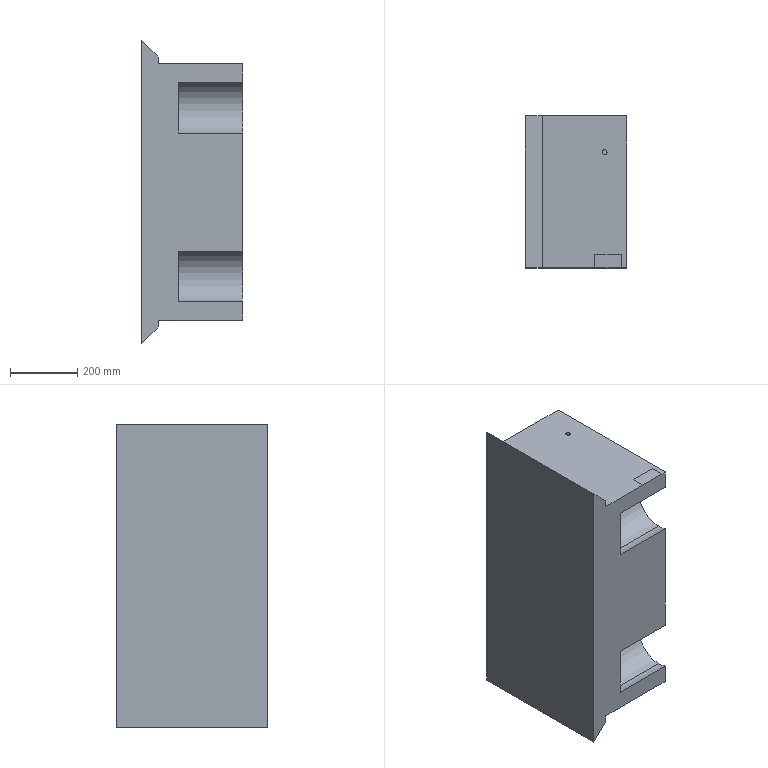Part | SolidWorks | features BaseBody 1 | 1 solid | 86 faces | box 300 x 450 x 900 mm | volume 94683231 mm3 | plane 38 | cylinder 30 | cone 16 | spline 2 | commonest cylinder face diameters 3.3 x16 14 x4 140 x4 160.037 x3 161.988 x3